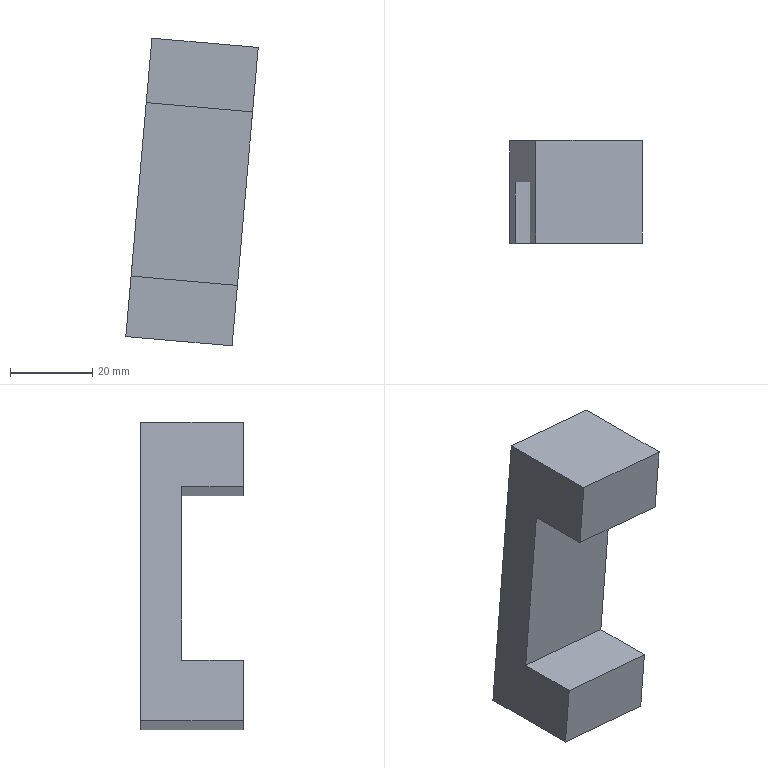Part | NX | features solid 2 | 1 solid | 10 faces | box 32.259 x 25 x 74.943 mm | volume 30874 mm3 | plane 10
STEP:
#1=CARTESIAN_POINT('',(-946.053,260.,-193.67));
#2=VERTEX_POINT('',#1);
#3=CARTESIAN_POINT('',(-949.75,260.,-235.934));
#4=VERTEX_POINT('',#3);
#5=CARTESIAN_POINT('',(-944.937,260.,-180.916));
#6=DIRECTION('',(-0.08716,0.,-0.9962));
#7=VECTOR('',#6,1000.);
#8=LINE('',#5,#7);
#9=EDGE_CURVE('',#2,#4,#8,.T.);
#10=ORIENTED_EDGE('',*,*,#9,.F.);
#11=CARTESIAN_POINT('',(-971.954,260.,-191.404));
#12=VERTEX_POINT('',#11);
#13=CARTESIAN_POINT('',(-959.003,260.,-192.537));
#14=DIRECTION('',(0.9962,0.,-0.08716));
#15=VECTOR('',#14,1000.);
#16=LINE('',#13,#15);
#17=EDGE_CURVE('',#2,#12,#16,.F.);
#18=ORIENTED_EDGE('',*,*,#17,.T.);
#19=CARTESIAN_POINT('',(-975.651,260.,-233.668));
#20=VERTEX_POINT('',#19);
#21=CARTESIAN_POINT('',(-970.838,260.,-178.65));
#22=DIRECTION('',(-0.08716,0.,-0.9962));
#23=VECTOR('',#22,1000.);
#24=LINE('',#21,#23);
#25=EDGE_CURVE('',#12,#20,#24,.T.);
#26=ORIENTED_EDGE('',*,*,#25,.T.);
#27=CARTESIAN_POINT('',(-947.155,260.,-236.161));
#28=DIRECTION('',(-0.9962,0.,0.08716));
#29=VECTOR('',#28,1000.);
#30=LINE('',#27,#29);
#31=EDGE_CURVE('',#4,#20,#30,.T.);
#32=ORIENTED_EDGE('',*,*,#31,.F.);
#33=EDGE_LOOP('',(#10,#18,#26,#32));
#34=FACE_BOUND('',#33,.T.);
#35=CARTESIAN_POINT('',(-957.887,260.,-179.783));
#36=DIRECTION('',(0.,-1.,0.));
#37=DIRECTION('',(-0.08716,0.,-0.9962));
#38=AXIS2_PLACEMENT_3D('',#35,#36,#37);
#39=PLANE('',#38);
#40=ADVANCED_FACE('',(#34),#39,.T.);
#41=ORIENTED_EDGE('',*,*,#25,.F.);
#42=CARTESIAN_POINT('',(-971.954,245.,-191.404));
#43=VERTEX_POINT('',#42);
#44=CARTESIAN_POINT('',(-971.954,260.,-191.404));
#45=DIRECTION('',(0.,-1.,0.));
#46=VECTOR('',#45,1000.);
#47=LINE('',#44,#46);
#48=EDGE_CURVE('',#12,#43,#47,.T.);
#49=ORIENTED_EDGE('',*,*,#48,.T.);
#50=CARTESIAN_POINT('',(-970.58,245.,-175.707));
#51=VERTEX_POINT('',#50);
#52=CARTESIAN_POINT('',(-971.954,245.,-191.404));
#53=DIRECTION('',(-0.08716,0.,-0.9962));
#54=VECTOR('',#53,1000.);
#55=LINE('',#52,#54);
#56=EDGE_CURVE('',#43,#51,#55,.F.);
#57=ORIENTED_EDGE('',*,*,#56,.T.);
#58=CARTESIAN_POINT('',(-970.58,270.,-175.707));
#59=VERTEX_POINT('',#58);
#60=CARTESIAN_POINT('',(-970.58,270.,-175.707));
#61=DIRECTION('',(0.,1.,0.));
#62=VECTOR('',#61,1000.);
#63=LINE('',#60,#62);
#64=EDGE_CURVE('',#59,#51,#63,.F.);
#65=ORIENTED_EDGE('',*,*,#64,.F.);
#66=CARTESIAN_POINT('',(-976.939,270.,-248.384));
#67=VERTEX_POINT('',#66);
#68=CARTESIAN_POINT('',(-970.838,270.,-178.65));
#69=DIRECTION('',(-0.08716,0.,-0.9962));
#70=VECTOR('',#69,1000.);
#71=LINE('',#68,#70);
#72=EDGE_CURVE('',#59,#67,#71,.T.);
#73=ORIENTED_EDGE('',*,*,#72,.T.);
#74=CARTESIAN_POINT('',(-976.939,245.,-248.384));
#75=VERTEX_POINT('',#74);
#76=CARTESIAN_POINT('',(-976.939,260.,-248.384));
#77=DIRECTION('',(0.,1.,0.));
#78=VECTOR('',#77,1000.);
#79=LINE('',#76,#78);
#80=EDGE_CURVE('',#75,#67,#79,.T.);
#81=ORIENTED_EDGE('',*,*,#80,.F.);
#82=CARTESIAN_POINT('',(-975.651,245.,-233.668));
#83=VERTEX_POINT('',#82);
#84=CARTESIAN_POINT('',(-976.939,245.,-248.384));
#85=DIRECTION('',(-0.08716,0.,-0.9962));
#86=VECTOR('',#85,1000.);
#87=LINE('',#84,#86);
#88=EDGE_CURVE('',#75,#83,#87,.F.);
#89=ORIENTED_EDGE('',*,*,#88,.T.);
#90=CARTESIAN_POINT('',(-975.651,260.,-233.668));
#91=DIRECTION('',(0.,1.,0.));
#92=VECTOR('',#91,1000.);
#93=LINE('',#90,#92);
#94=EDGE_CURVE('',#20,#83,#93,.F.);
#95=ORIENTED_EDGE('',*,*,#94,.F.);
#96=EDGE_LOOP('',(#41,#49,#57,#65,#73,#81,#89,#95));
#97=FACE_BOUND('',#96,.T.);
#98=CARTESIAN_POINT('',(-970.838,260.,-178.65));
#99=DIRECTION('',(-0.9962,0.,0.08716));
#100=DIRECTION('',(-0.08716,0.,-0.9962));
#101=AXIS2_PLACEMENT_3D('',#98,#99,#100);
#102=PLANE('',#101);
#103=ADVANCED_FACE('',(#97),#102,.T.);
#104=CARTESIAN_POINT('',(-951.038,245.,-250.65));
#105=VERTEX_POINT('',#104);
#106=CARTESIAN_POINT('',(-951.038,270.,-250.65));
#107=VERTEX_POINT('',#106);
#108=CARTESIAN_POINT('',(-951.038,260.,-250.65));
#109=DIRECTION('',(0.,1.,0.));
#110=VECTOR('',#109,1000.);
#111=LINE('',#108,#110);
#112=EDGE_CURVE('',#105,#107,#111,.T.);
#113=ORIENTED_EDGE('',*,*,#112,.F.);
#114=CARTESIAN_POINT('',(-951.038,245.,-250.65));
#115=DIRECTION('',(-0.9962,0.,0.08716));
#116=VECTOR('',#115,1000.);
#117=LINE('',#114,#116);
#118=EDGE_CURVE('',#105,#75,#117,.T.);
#119=ORIENTED_EDGE('',*,*,#118,.T.);
#120=ORIENTED_EDGE('',*,*,#80,.T.);
#121=CARTESIAN_POINT('',(-963.988,270.,-249.517));
#122=DIRECTION('',(-0.9962,0.,0.08716));
#123=VECTOR('',#122,1000.);
#124=LINE('',#121,#123);
#125=EDGE_CURVE('',#107,#67,#124,.T.);
#126=ORIENTED_EDGE('',*,*,#125,.F.);
#127=EDGE_LOOP('',(#113,#119,#120,#126));
#128=FACE_BOUND('',#127,.T.);
#129=CARTESIAN_POINT('',(-963.988,260.,-249.517));
#130=DIRECTION('',(-0.08716,0.,-0.9962));
#131=DIRECTION('',(0.,1.,0.));
#132=AXIS2_PLACEMENT_3D('',#129,#130,#131);
#133=PLANE('',#132);
#134=ADVANCED_FACE('',(#128),#133,.T.);
#135=ORIENTED_EDGE('',*,*,#72,.F.);
#136=CARTESIAN_POINT('',(-944.679,270.,-177.973));
#137=VERTEX_POINT('',#136);
#138=CARTESIAN_POINT('',(-944.16,270.,-178.019));
#139=DIRECTION('',(-0.9962,0.,0.08716));
#140=VECTOR('',#139,1000.);
#141=LINE('',#138,#140);
#142=EDGE_CURVE('',#137,#59,#141,.T.);
#143=ORIENTED_EDGE('',*,*,#142,.F.);
#144=CARTESIAN_POINT('',(-944.937,270.,-180.916));
#145=DIRECTION('',(-0.08716,0.,-0.9962));
#146=VECTOR('',#145,1000.);
#147=LINE('',#144,#146);
#148=EDGE_CURVE('',#137,#107,#147,.T.);
#149=ORIENTED_EDGE('',*,*,#148,.T.);
#150=ORIENTED_EDGE('',*,*,#125,.T.);
#151=EDGE_LOOP('',(#135,#143,#149,#150));
#152=FACE_BOUND('',#151,.T.);
#153=CARTESIAN_POINT('',(-957.887,270.,-179.783));
#154=DIRECTION('',(0.,-1.,0.));
#155=DIRECTION('',(-0.08716,0.,-0.9962));
#156=AXIS2_PLACEMENT_3D('',#153,#154,#155);
#157=PLANE('',#156);
#158=ADVANCED_FACE('',(#152),#157,.F.);
#159=CARTESIAN_POINT('',(-946.053,245.,-193.67));
#160=VERTEX_POINT('',#159);
#161=CARTESIAN_POINT('',(-946.053,260.,-193.67));
#162=DIRECTION('',(0.,-1.,0.));
#163=VECTOR('',#162,1000.);
#164=LINE('',#161,#163);
#165=EDGE_CURVE('',#2,#160,#164,.T.);
#166=ORIENTED_EDGE('',*,*,#165,.F.);
#167=ORIENTED_EDGE('',*,*,#9,.T.);
#168=CARTESIAN_POINT('',(-949.75,245.,-235.934));
#169=VERTEX_POINT('',#168);
#170=CARTESIAN_POINT('',(-949.75,260.,-235.934));
#171=DIRECTION('',(0.,1.,0.));
#172=VECTOR('',#171,1000.);
#173=LINE('',#170,#172);
#174=EDGE_CURVE('',#4,#169,#173,.F.);
#175=ORIENTED_EDGE('',*,*,#174,.T.);
#176=CARTESIAN_POINT('',(-951.038,245.,-250.65));
#177=DIRECTION('',(-0.08716,0.,-0.9962));
#178=VECTOR('',#177,1000.);
#179=LINE('',#176,#178);
#180=EDGE_CURVE('',#105,#169,#179,.F.);
#181=ORIENTED_EDGE('',*,*,#180,.F.);
#182=ORIENTED_EDGE('',*,*,#112,.T.);
#183=ORIENTED_EDGE('',*,*,#148,.F.);
#184=CARTESIAN_POINT('',(-944.679,245.,-177.973));
#185=VERTEX_POINT('',#184);
#186=CARTESIAN_POINT('',(-944.679,270.,-177.973));
#187=DIRECTION('',(0.,1.,0.));
#188=VECTOR('',#187,1000.);
#189=LINE('',#186,#188);
#190=EDGE_CURVE('',#137,#185,#189,.F.);
#191=ORIENTED_EDGE('',*,*,#190,.T.);
#192=CARTESIAN_POINT('',(-946.053,245.,-193.67));
#193=DIRECTION('',(-0.08716,0.,-0.9962));
#194=VECTOR('',#193,1000.);
#195=LINE('',#192,#194);
#196=EDGE_CURVE('',#160,#185,#195,.F.);
#197=ORIENTED_EDGE('',*,*,#196,.F.);
#198=EDGE_LOOP('',(#166,#167,#175,#181,#182,#183,#191,#197));
#199=FACE_BOUND('',#198,.T.);
#200=CARTESIAN_POINT('',(-944.937,260.,-180.916));
#201=DIRECTION('',(-0.9962,0.,0.08716));
#202=DIRECTION('',(-0.08716,0.,-0.9962));
#203=AXIS2_PLACEMENT_3D('',#200,#201,#202);
#204=PLANE('',#203);
#205=ADVANCED_FACE('',(#199),#204,.F.);
#206=ORIENTED_EDGE('',*,*,#174,.F.);
#207=ORIENTED_EDGE('',*,*,#31,.T.);
#208=ORIENTED_EDGE('',*,*,#94,.T.);
#209=CARTESIAN_POINT('',(-947.155,245.,-236.161));
#210=DIRECTION('',(-0.9962,0.,0.08716));
#211=VECTOR('',#210,1000.);
#212=LINE('',#209,#211);
#213=EDGE_CURVE('',#169,#83,#212,.T.);
#214=ORIENTED_EDGE('',*,*,#213,.F.);
#215=EDGE_LOOP('',(#206,#207,#208,#214));
#216=FACE_BOUND('',#215,.T.);
#217=CARTESIAN_POINT('',(-947.155,260.,-236.161));
#218=DIRECTION('',(-0.08716,0.,-0.9962));
#219=DIRECTION('',(-0.9962,0.,0.08716));
#220=AXIS2_PLACEMENT_3D('',#217,#218,#219);
#221=PLANE('',#220);
#222=ADVANCED_FACE('',(#216),#221,.F.);
#223=ORIENTED_EDGE('',*,*,#213,.T.);
#224=ORIENTED_EDGE('',*,*,#88,.F.);
#225=ORIENTED_EDGE('',*,*,#118,.F.);
#226=ORIENTED_EDGE('',*,*,#180,.T.);
#227=EDGE_LOOP('',(#223,#224,#225,#226));
#228=FACE_BOUND('',#227,.T.);
#229=CARTESIAN_POINT('',(-951.038,245.,-250.65));
#230=DIRECTION('',(0.,-1.,0.));
#231=DIRECTION('',(-1.,0.,0.));
#232=AXIS2_PLACEMENT_3D('',#229,#230,#231);
#233=PLANE('',#232);
#234=ADVANCED_FACE('',(#228),#233,.T.);
#235=ORIENTED_EDGE('',*,*,#17,.F.);
#236=ORIENTED_EDGE('',*,*,#165,.T.);
#237=CARTESIAN_POINT('',(-948.301,245.,-193.474));
#238=DIRECTION('',(-0.9962,0.,0.08716));
#239=VECTOR('',#238,1000.);
#240=LINE('',#237,#239);
#241=EDGE_CURVE('',#160,#43,#240,.T.);
#242=ORIENTED_EDGE('',*,*,#241,.T.);
#243=ORIENTED_EDGE('',*,*,#48,.F.);
#244=EDGE_LOOP('',(#235,#236,#242,#243));
#245=FACE_BOUND('',#244,.T.);
#246=CARTESIAN_POINT('',(-948.301,270.,-193.474));
#247=DIRECTION('',(-0.08716,0.,-0.9962));
#248=DIRECTION('',(-0.9962,0.,0.08716));
#249=AXIS2_PLACEMENT_3D('',#246,#247,#248);
#250=PLANE('',#249);
#251=ADVANCED_FACE('',(#245),#250,.T.);
#252=ORIENTED_EDGE('',*,*,#190,.F.);
#253=ORIENTED_EDGE('',*,*,#142,.T.);
#254=ORIENTED_EDGE('',*,*,#64,.T.);
#255=CARTESIAN_POINT('',(-944.16,245.,-178.019));
#256=DIRECTION('',(-0.9962,0.,0.08716));
#257=VECTOR('',#256,1000.);
#258=LINE('',#255,#257);
#259=EDGE_CURVE('',#185,#51,#258,.T.);
#260=ORIENTED_EDGE('',*,*,#259,.F.);
#261=EDGE_LOOP('',(#252,#253,#254,#260));
#262=FACE_BOUND('',#261,.T.);
#263=CARTESIAN_POINT('',(-944.16,270.,-178.019));
#264=DIRECTION('',(-0.08716,0.,-0.9962));
#265=DIRECTION('',(-0.9962,0.,0.08716));
#266=AXIS2_PLACEMENT_3D('',#263,#264,#265);
#267=PLANE('',#266);
#268=ADVANCED_FACE('',(#262),#267,.F.);
#269=ORIENTED_EDGE('',*,*,#259,.T.);
#270=ORIENTED_EDGE('',*,*,#56,.F.);
#271=ORIENTED_EDGE('',*,*,#241,.F.);
#272=ORIENTED_EDGE('',*,*,#196,.T.);
#273=EDGE_LOOP('',(#269,#270,#271,#272));
#274=FACE_BOUND('',#273,.T.);
#275=CARTESIAN_POINT('',(-948.301,245.,-193.474));
#276=DIRECTION('',(0.,-1.,0.));
#277=DIRECTION('',(-1.,0.,0.));
#278=AXIS2_PLACEMENT_3D('',#275,#276,#277);
#279=PLANE('',#278);
#280=ADVANCED_FACE('',(#274),#279,.T.);
#281=CLOSED_SHELL('',(#40,#103,#134,#158,#205,#222,#234,#251,#268,#280));
#282=MANIFOLD_SOLID_BREP('',#281);
#283=(LENGTH_UNIT()NAMED_UNIT(*)SI_UNIT(.MILLI.,.METRE.));
#284=UNCERTAINTY_MEASURE_WITH_UNIT(LENGTH_MEASURE(0.00001),#283,'','');
#285=(NAMED_UNIT(*)PLANE_ANGLE_UNIT()SI_UNIT($,.RADIAN.));
#286=(NAMED_UNIT(*)SI_UNIT($,.STERADIAN.)SOLID_ANGLE_UNIT());
#287=(GEOMETRIC_REPRESENTATION_CONTEXT(3)GLOBAL_UNCERTAINTY_ASSIGNED_CONTEXT((#284))GLOBAL_UNIT_ASSIGNED_CONTEXT((#283,#285,#286))REPRESENTATION_CONTEXT('',''));
#288=ADVANCED_BREP_SHAPE_REPRESENTATION('',(#282),#287);